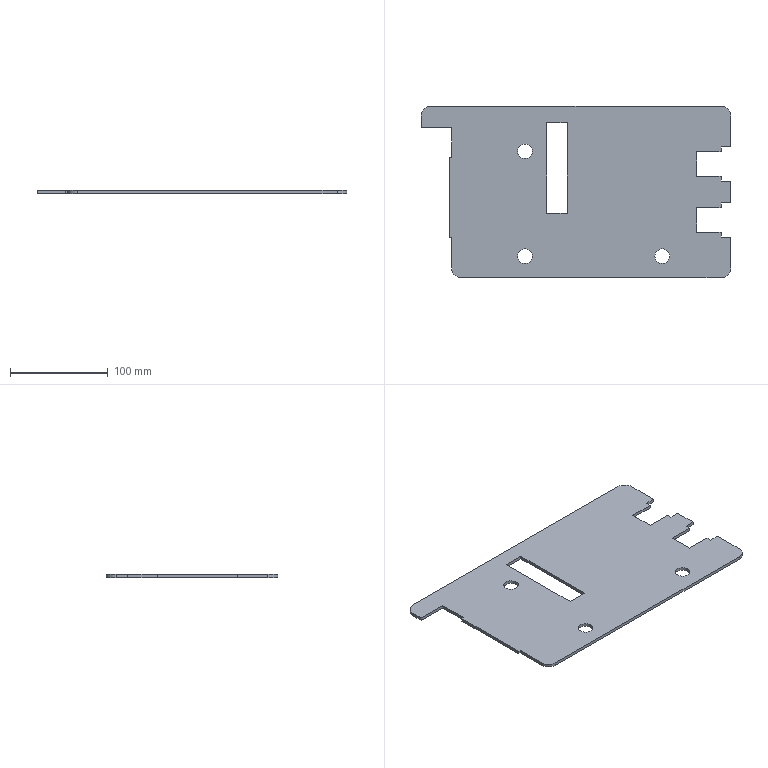Part | SolidWorks | features FlatPattern 1, SMBaseFlange 1, SheetMetal 1 | 1 solid | 42 faces | box 316 x 175 x 3.2 mm | volume 147992 mm3 | plane 32 | cylinder 10 | commonest cylinder face diameters 15 x6 20 x4
STEP:
#1=CARTESIAN_POINT('',(-77.5,-136.,3.2));
#2=VERTEX_POINT('',#1);
#3=CARTESIAN_POINT('',(-62.5,-136.,3.2));
#4=VERTEX_POINT('',#3);
#5=CARTESIAN_POINT('',(-70.,-136.,3.2));
#6=DIRECTION('',(0.,0.,1.));
#7=DIRECTION('',(1.,0.,0.));
#8=AXIS2_PLACEMENT_3D('',#5,#6,#7);
#9=CIRCLE('',#8,7.5);
#10=EDGE_CURVE('',#2,#4,#9,.T.);
#11=ORIENTED_EDGE('',*,*,#10,.T.);
#12=CARTESIAN_POINT('',(-62.5,-136.,0.));
#13=VERTEX_POINT('',#12);
#14=CARTESIAN_POINT('',(-62.5,-136.,3.2));
#15=DIRECTION('',(0.,0.,-1.));
#16=VECTOR('',#15,1000.);
#17=LINE('',#14,#16);
#18=EDGE_CURVE('',#4,#13,#17,.T.);
#19=ORIENTED_EDGE('',*,*,#18,.T.);
#20=CARTESIAN_POINT('',(-77.5,-136.,0.));
#21=VERTEX_POINT('',#20);
#22=CARTESIAN_POINT('',(-70.,-136.,0.));
#23=DIRECTION('',(0.,0.,1.));
#24=DIRECTION('',(1.,0.,0.));
#25=AXIS2_PLACEMENT_3D('',#22,#23,#24);
#26=CIRCLE('',#25,7.5);
#27=EDGE_CURVE('',#21,#13,#26,.T.);
#28=ORIENTED_EDGE('',*,*,#27,.F.);
#29=CARTESIAN_POINT('',(-77.5,-136.,3.2));
#30=DIRECTION('',(0.,0.,-1.));
#31=VECTOR('',#30,1000.);
#32=LINE('',#29,#31);
#33=EDGE_CURVE('',#2,#21,#32,.T.);
#34=ORIENTED_EDGE('',*,*,#33,.F.);
#35=EDGE_LOOP('',(#11,#19,#28,#34));
#36=FACE_OUTER_BOUND('',#35,.T.);
#37=CARTESIAN_POINT('',(-70.,-136.,3.2));
#38=DIRECTION('',(0.,0.,-1.));
#39=DIRECTION('',(-1.,0.,0.));
#40=AXIS2_PLACEMENT_3D('',#37,#38,#39);
#41=CYLINDRICAL_SURFACE('',#40,7.5);
#42=ADVANCED_FACE('',(#36),#41,.F.);
#43=CARTESIAN_POINT('',(-217.5,-136.,3.2));
#44=VERTEX_POINT('',#43);
#45=CARTESIAN_POINT('',(-202.5,-136.,3.2));
#46=VERTEX_POINT('',#45);
#47=CARTESIAN_POINT('',(-210.,-136.,3.2));
#48=DIRECTION('',(0.,0.,1.));
#49=DIRECTION('',(1.,0.,0.));
#50=AXIS2_PLACEMENT_3D('',#47,#48,#49);
#51=CIRCLE('',#50,7.5);
#52=EDGE_CURVE('',#44,#46,#51,.T.);
#53=ORIENTED_EDGE('',*,*,#52,.T.);
#54=CARTESIAN_POINT('',(-202.5,-136.,0.));
#55=VERTEX_POINT('',#54);
#56=CARTESIAN_POINT('',(-202.5,-136.,3.2));
#57=DIRECTION('',(0.,0.,-1.));
#58=VECTOR('',#57,1000.);
#59=LINE('',#56,#58);
#60=EDGE_CURVE('',#46,#55,#59,.T.);
#61=ORIENTED_EDGE('',*,*,#60,.T.);
#62=CARTESIAN_POINT('',(-217.5,-136.,0.));
#63=VERTEX_POINT('',#62);
#64=CARTESIAN_POINT('',(-210.,-136.,0.));
#65=DIRECTION('',(0.,0.,1.));
#66=DIRECTION('',(1.,0.,0.));
#67=AXIS2_PLACEMENT_3D('',#64,#65,#66);
#68=CIRCLE('',#67,7.5);
#69=EDGE_CURVE('',#63,#55,#68,.T.);
#70=ORIENTED_EDGE('',*,*,#69,.F.);
#71=CARTESIAN_POINT('',(-217.5,-136.,3.2));
#72=DIRECTION('',(0.,0.,-1.));
#73=VECTOR('',#72,1000.);
#74=LINE('',#71,#73);
#75=EDGE_CURVE('',#44,#63,#74,.T.);
#76=ORIENTED_EDGE('',*,*,#75,.F.);
#77=EDGE_LOOP('',(#53,#61,#70,#76));
#78=FACE_OUTER_BOUND('',#77,.T.);
#79=CARTESIAN_POINT('',(-210.,-136.,3.2));
#80=DIRECTION('',(0.,0.,-1.));
#81=DIRECTION('',(-1.,0.,0.));
#82=AXIS2_PLACEMENT_3D('',#79,#80,#81);
#83=CYLINDRICAL_SURFACE('',#82,7.5);
#84=ADVANCED_FACE('',(#78),#83,.F.);
#85=CARTESIAN_POINT('',(-217.5,-29.,3.2));
#86=VERTEX_POINT('',#85);
#87=CARTESIAN_POINT('',(-202.5,-29.,3.2));
#88=VERTEX_POINT('',#87);
#89=CARTESIAN_POINT('',(-210.,-29.,3.2));
#90=DIRECTION('',(0.,0.,1.));
#91=DIRECTION('',(1.,0.,0.));
#92=AXIS2_PLACEMENT_3D('',#89,#90,#91);
#93=CIRCLE('',#92,7.5);
#94=EDGE_CURVE('',#86,#88,#93,.T.);
#95=ORIENTED_EDGE('',*,*,#94,.T.);
#96=CARTESIAN_POINT('',(-202.5,-29.,0.));
#97=VERTEX_POINT('',#96);
#98=CARTESIAN_POINT('',(-202.5,-29.,3.2));
#99=DIRECTION('',(0.,0.,-1.));
#100=VECTOR('',#99,1000.);
#101=LINE('',#98,#100);
#102=EDGE_CURVE('',#88,#97,#101,.T.);
#103=ORIENTED_EDGE('',*,*,#102,.T.);
#104=CARTESIAN_POINT('',(-217.5,-29.,0.));
#105=VERTEX_POINT('',#104);
#106=CARTESIAN_POINT('',(-210.,-29.,0.));
#107=DIRECTION('',(0.,0.,1.));
#108=DIRECTION('',(1.,0.,0.));
#109=AXIS2_PLACEMENT_3D('',#106,#107,#108);
#110=CIRCLE('',#109,7.5);
#111=EDGE_CURVE('',#105,#97,#110,.T.);
#112=ORIENTED_EDGE('',*,*,#111,.F.);
#113=CARTESIAN_POINT('',(-217.5,-29.,3.2));
#114=DIRECTION('',(0.,0.,-1.));
#115=VECTOR('',#114,1000.);
#116=LINE('',#113,#115);
#117=EDGE_CURVE('',#86,#105,#116,.T.);
#118=ORIENTED_EDGE('',*,*,#117,.F.);
#119=EDGE_LOOP('',(#95,#103,#112,#118));
#120=FACE_OUTER_BOUND('',#119,.T.);
#121=CARTESIAN_POINT('',(-210.,-29.,3.2));
#122=DIRECTION('',(0.,0.,-1.));
#123=DIRECTION('',(-1.,0.,0.));
#124=AXIS2_PLACEMENT_3D('',#121,#122,#123);
#125=CYLINDRICAL_SURFACE('',#124,7.5);
#126=ADVANCED_FACE('',(#120),#125,.F.);
#127=ORIENTED_EDGE('',*,*,#10,.F.);
#128=CARTESIAN_POINT('',(-70.,-136.,3.2));
#129=DIRECTION('',(0.,0.,1.));
#130=DIRECTION('',(1.,0.,0.));
#131=AXIS2_PLACEMENT_3D('',#128,#129,#130);
#132=CIRCLE('',#131,7.5);
#133=EDGE_CURVE('',#4,#2,#132,.T.);
#134=ORIENTED_EDGE('',*,*,#133,.F.);
#135=EDGE_LOOP('',(#127,#134));
#136=FACE_BOUND('',#135,.T.);
#137=ORIENTED_EDGE('',*,*,#52,.F.);
#138=CARTESIAN_POINT('',(-210.,-136.,3.2));
#139=DIRECTION('',(0.,0.,1.));
#140=DIRECTION('',(1.,0.,0.));
#141=AXIS2_PLACEMENT_3D('',#138,#139,#140);
#142=CIRCLE('',#141,7.5);
#143=EDGE_CURVE('',#46,#44,#142,.T.);
#144=ORIENTED_EDGE('',*,*,#143,.F.);
#145=EDGE_LOOP('',(#137,#144));
#146=FACE_BOUND('',#145,.T.);
#147=ORIENTED_EDGE('',*,*,#94,.F.);
#148=CARTESIAN_POINT('',(-210.,-29.,3.2));
#149=DIRECTION('',(0.,0.,1.));
#150=DIRECTION('',(1.,0.,0.));
#151=AXIS2_PLACEMENT_3D('',#148,#149,#150);
#152=CIRCLE('',#151,7.5);
#153=EDGE_CURVE('',#88,#86,#152,.T.);
#154=ORIENTED_EDGE('',*,*,#153,.F.);
#155=EDGE_LOOP('',(#147,#154));
#156=FACE_BOUND('',#155,.T.);
#157=CARTESIAN_POINT('',(-285.,-148.,3.2));
#158=VERTEX_POINT('',#157);
#159=CARTESIAN_POINT('',(-275.,-158.,3.2));
#160=VERTEX_POINT('',#159);
#161=CARTESIAN_POINT('',(-275.,-148.,3.2));
#162=DIRECTION('',(0.,0.,1.));
#163=DIRECTION('',(-1.,0.,0.));
#164=AXIS2_PLACEMENT_3D('',#161,#162,#163);
#165=CIRCLE('',#164,10.);
#166=EDGE_CURVE('',#158,#160,#165,.T.);
#167=ORIENTED_EDGE('',*,*,#166,.T.);
#168=CARTESIAN_POINT('',(-10.,-158.,3.2));
#169=VERTEX_POINT('',#168);
#170=CARTESIAN_POINT('',(-275.,-158.,3.2));
#171=DIRECTION('',(1.,0.,0.));
#172=VECTOR('',#171,1000.);
#173=LINE('',#170,#172);
#174=EDGE_CURVE('',#160,#169,#173,.T.);
#175=ORIENTED_EDGE('',*,*,#174,.T.);
#176=CARTESIAN_POINT('',(0.,-148.,3.2));
#177=VERTEX_POINT('',#176);
#178=CARTESIAN_POINT('',(-10.,-148.,3.2));
#179=DIRECTION('',(0.,0.,1.));
#180=DIRECTION('',(1.,0.,0.));
#181=AXIS2_PLACEMENT_3D('',#178,#179,#180);
#182=CIRCLE('',#181,10.);
#183=EDGE_CURVE('',#169,#177,#182,.T.);
#184=ORIENTED_EDGE('',*,*,#183,.T.);
#185=CARTESIAN_POINT('',(0.,-116.5,3.2));
#186=VERTEX_POINT('',#185);
#187=CARTESIAN_POINT('',(0.,-148.,3.2));
#188=DIRECTION('',(0.,1.,0.));
#189=VECTOR('',#188,1000.);
#190=LINE('',#187,#189);
#191=EDGE_CURVE('',#177,#186,#190,.T.);
#192=ORIENTED_EDGE('',*,*,#191,.T.);
#193=CARTESIAN_POINT('',(-10.,-116.5,3.2));
#194=VERTEX_POINT('',#193);
#195=CARTESIAN_POINT('',(-10.,-116.5,3.2));
#196=DIRECTION('',(-1.,0.,0.));
#197=VECTOR('',#196,1000.);
#198=LINE('',#195,#197);
#199=EDGE_CURVE('',#186,#194,#198,.T.);
#200=ORIENTED_EDGE('',*,*,#199,.T.);
#201=CARTESIAN_POINT('',(-10.,-111.5,3.2));
#202=VERTEX_POINT('',#201);
#203=CARTESIAN_POINT('',(-10.,-111.5,3.2));
#204=DIRECTION('',(0.,1.,0.));
#205=VECTOR('',#204,1000.);
#206=LINE('',#203,#205);
#207=EDGE_CURVE('',#194,#202,#206,.T.);
#208=ORIENTED_EDGE('',*,*,#207,.T.);
#209=CARTESIAN_POINT('',(-35.,-111.5,3.2));
#210=VERTEX_POINT('',#209);
#211=CARTESIAN_POINT('',(-35.,-111.5,3.2));
#212=DIRECTION('',(-1.,0.,0.));
#213=VECTOR('',#212,1000.);
#214=LINE('',#211,#213);
#215=EDGE_CURVE('',#202,#210,#214,.T.);
#216=ORIENTED_EDGE('',*,*,#215,.T.);
#217=CARTESIAN_POINT('',(-35.,-86.5,3.2));
#218=VERTEX_POINT('',#217);
#219=CARTESIAN_POINT('',(-35.,-111.5,3.2));
#220=DIRECTION('',(0.,1.,0.));
#221=VECTOR('',#220,1000.);
#222=LINE('',#219,#221);
#223=EDGE_CURVE('',#210,#218,#222,.T.);
#224=ORIENTED_EDGE('',*,*,#223,.T.);
#225=CARTESIAN_POINT('',(-10.,-86.5,3.2));
#226=VERTEX_POINT('',#225);
#227=CARTESIAN_POINT('',(-35.,-86.5,3.2));
#228=DIRECTION('',(1.,0.,0.));
#229=VECTOR('',#228,1000.);
#230=LINE('',#227,#229);
#231=EDGE_CURVE('',#218,#226,#230,.T.);
#232=ORIENTED_EDGE('',*,*,#231,.T.);
#233=CARTESIAN_POINT('',(-10.,-81.5,3.2));
#234=VERTEX_POINT('',#233);
#235=CARTESIAN_POINT('',(-10.,-86.5,3.2));
#236=DIRECTION('',(0.,1.,0.));
#237=VECTOR('',#236,1000.);
#238=LINE('',#235,#237);
#239=EDGE_CURVE('',#226,#234,#238,.T.);
#240=ORIENTED_EDGE('',*,*,#239,.T.);
#241=CARTESIAN_POINT('',(0.,-81.5,3.2));
#242=VERTEX_POINT('',#241);
#243=CARTESIAN_POINT('',(-10.,-81.5,3.2));
#244=DIRECTION('',(1.,0.,0.));
#245=VECTOR('',#244,1000.);
#246=LINE('',#243,#245);
#247=EDGE_CURVE('',#234,#242,#246,.T.);
#248=ORIENTED_EDGE('',*,*,#247,.T.);
#249=CARTESIAN_POINT('',(0.,-59.5,3.2));
#250=VERTEX_POINT('',#249);
#251=CARTESIAN_POINT('',(0.,-81.5,3.2));
#252=DIRECTION('',(0.,1.,0.));
#253=VECTOR('',#252,1000.);
#254=LINE('',#251,#253);
#255=EDGE_CURVE('',#242,#250,#254,.T.);
#256=ORIENTED_EDGE('',*,*,#255,.T.);
#257=CARTESIAN_POINT('',(-10.,-59.5,3.2));
#258=VERTEX_POINT('',#257);
#259=CARTESIAN_POINT('',(-10.,-59.5,3.2));
#260=DIRECTION('',(-1.,0.,0.));
#261=VECTOR('',#260,1000.);
#262=LINE('',#259,#261);
#263=EDGE_CURVE('',#250,#258,#262,.T.);
#264=ORIENTED_EDGE('',*,*,#263,.T.);
#265=CARTESIAN_POINT('',(-10.,-54.5,3.2));
#266=VERTEX_POINT('',#265);
#267=CARTESIAN_POINT('',(-10.,-54.5,3.2));
#268=DIRECTION('',(0.,1.,0.));
#269=VECTOR('',#268,1000.);
#270=LINE('',#267,#269);
#271=EDGE_CURVE('',#258,#266,#270,.T.);
#272=ORIENTED_EDGE('',*,*,#271,.T.);
#273=CARTESIAN_POINT('',(-35.,-54.5,3.2));
#274=VERTEX_POINT('',#273);
#275=CARTESIAN_POINT('',(-35.,-54.5,3.2));
#276=DIRECTION('',(-1.,0.,0.));
#277=VECTOR('',#276,1000.);
#278=LINE('',#275,#277);
#279=EDGE_CURVE('',#266,#274,#278,.T.);
#280=ORIENTED_EDGE('',*,*,#279,.T.);
#281=CARTESIAN_POINT('',(-35.,-29.5,3.2));
#282=VERTEX_POINT('',#281);
#283=CARTESIAN_POINT('',(-35.,-54.5,3.2));
#284=DIRECTION('',(0.,1.,0.));
#285=VECTOR('',#284,1000.);
#286=LINE('',#283,#285);
#287=EDGE_CURVE('',#274,#282,#286,.T.);
#288=ORIENTED_EDGE('',*,*,#287,.T.);
#289=CARTESIAN_POINT('',(-10.,-29.5,3.2));
#290=VERTEX_POINT('',#289);
#291=CARTESIAN_POINT('',(-35.,-29.5,3.2));
#292=DIRECTION('',(1.,0.,0.));
#293=VECTOR('',#292,1000.);
#294=LINE('',#291,#293);
#295=EDGE_CURVE('',#282,#290,#294,.T.);
#296=ORIENTED_EDGE('',*,*,#295,.T.);
#297=CARTESIAN_POINT('',(-10.,-24.5,3.2));
#298=VERTEX_POINT('',#297);
#299=CARTESIAN_POINT('',(-10.,-29.5,3.2));
#300=DIRECTION('',(0.,1.,0.));
#301=VECTOR('',#300,1000.);
#302=LINE('',#299,#301);
#303=EDGE_CURVE('',#290,#298,#302,.T.);
#304=ORIENTED_EDGE('',*,*,#303,.T.);
#305=CARTESIAN_POINT('',(0.,-24.5,3.2));
#306=VERTEX_POINT('',#305);
#307=CARTESIAN_POINT('',(-10.,-24.5,3.2));
#308=DIRECTION('',(1.,0.,0.));
#309=VECTOR('',#308,1000.);
#310=LINE('',#307,#309);
#311=EDGE_CURVE('',#298,#306,#310,.T.);
#312=ORIENTED_EDGE('',*,*,#311,.T.);
#313=CARTESIAN_POINT('',(0.,7.,3.2));
#314=VERTEX_POINT('',#313);
#315=CARTESIAN_POINT('',(0.,-24.5,3.2));
#316=DIRECTION('',(0.,1.,0.));
#317=VECTOR('',#316,1000.);
#318=LINE('',#315,#317);
#319=EDGE_CURVE('',#306,#314,#318,.T.);
#320=ORIENTED_EDGE('',*,*,#319,.T.);
#321=CARTESIAN_POINT('',(-10.,17.,3.2));
#322=VERTEX_POINT('',#321);
#323=CARTESIAN_POINT('',(-10.,7.,3.2));
#324=DIRECTION('',(0.,0.,1.));
#325=DIRECTION('',(1.,0.,0.));
#326=AXIS2_PLACEMENT_3D('',#323,#324,#325);
#327=CIRCLE('',#326,10.);
#328=EDGE_CURVE('',#314,#322,#327,.T.);
#329=ORIENTED_EDGE('',*,*,#328,.T.);
#330=CARTESIAN_POINT('',(-306.,17.,3.2));
#331=VERTEX_POINT('',#330);
#332=CARTESIAN_POINT('',(-10.,17.,3.2));
#333=DIRECTION('',(-1.,0.,0.));
#334=VECTOR('',#333,1000.);
#335=LINE('',#332,#334);
#336=EDGE_CURVE('',#322,#331,#335,.T.);
#337=ORIENTED_EDGE('',*,*,#336,.T.);
#338=CARTESIAN_POINT('',(-316.,7.,3.2));
#339=VERTEX_POINT('',#338);
#340=CARTESIAN_POINT('',(-306.,7.,3.2));
#341=DIRECTION('',(0.,0.,1.));
#342=DIRECTION('',(1.,0.,0.));
#343=AXIS2_PLACEMENT_3D('',#340,#341,#342);
#344=CIRCLE('',#343,10.);
#345=EDGE_CURVE('',#331,#339,#344,.T.);
#346=ORIENTED_EDGE('',*,*,#345,.T.);
#347=CARTESIAN_POINT('',(-316.,-5.,3.2));
#348=VERTEX_POINT('',#347);
#349=CARTESIAN_POINT('',(-316.,7.,3.2));
#350=DIRECTION('',(0.,-1.,0.));
#351=VECTOR('',#350,1000.);
#352=LINE('',#349,#351);
#353=EDGE_CURVE('',#339,#348,#352,.T.);
#354=ORIENTED_EDGE('',*,*,#353,.T.);
#355=CARTESIAN_POINT('',(-285.,-5.,3.2));
#356=VERTEX_POINT('',#355);
#357=CARTESIAN_POINT('',(-316.,-5.,3.2));
#358=DIRECTION('',(1.,0.,0.));
#359=VECTOR('',#358,1000.);
#360=LINE('',#357,#359);
#361=EDGE_CURVE('',#348,#356,#360,.T.);
#362=ORIENTED_EDGE('',*,*,#361,.T.);
#363=CARTESIAN_POINT('',(-285.,-35.,3.2));
#364=VERTEX_POINT('',#363);
#365=CARTESIAN_POINT('',(-285.,-35.,3.2));
#366=DIRECTION('',(0.,-1.,0.));
#367=VECTOR('',#366,1000.);
#368=LINE('',#365,#367);
#369=EDGE_CURVE('',#356,#364,#368,.T.);
#370=ORIENTED_EDGE('',*,*,#369,.T.);
#371=CARTESIAN_POINT('',(-287.3,-35.,3.2));
#372=VERTEX_POINT('',#371);
#373=CARTESIAN_POINT('',(-285.,-35.,3.2));
#374=DIRECTION('',(-1.,0.,0.));
#375=VECTOR('',#374,1000.);
#376=LINE('',#373,#375);
#377=EDGE_CURVE('',#364,#372,#376,.T.);
#378=ORIENTED_EDGE('',*,*,#377,.T.);
#379=CARTESIAN_POINT('',(-287.3,-117.,3.2));
#380=VERTEX_POINT('',#379);
#381=CARTESIAN_POINT('',(-287.3,-35.,3.2));
#382=DIRECTION('',(0.,-1.,0.));
#383=VECTOR('',#382,1000.);
#384=LINE('',#381,#383);
#385=EDGE_CURVE('',#372,#380,#384,.T.);
#386=ORIENTED_EDGE('',*,*,#385,.T.);
#387=CARTESIAN_POINT('',(-285.,-117.,3.2));
#388=VERTEX_POINT('',#387);
#389=CARTESIAN_POINT('',(-287.3,-117.,3.2));
#390=DIRECTION('',(1.,0.,0.));
#391=VECTOR('',#390,1000.);
#392=LINE('',#389,#391);
#393=EDGE_CURVE('',#380,#388,#392,.T.);
#394=ORIENTED_EDGE('',*,*,#393,.T.);
#395=CARTESIAN_POINT('',(-285.,-148.,3.2));
#396=DIRECTION('',(0.,-1.,0.));
#397=VECTOR('',#396,1000.);
#398=LINE('',#395,#397);
#399=EDGE_CURVE('',#388,#158,#398,.T.);
#400=ORIENTED_EDGE('',*,*,#399,.T.);
#401=EDGE_LOOP('',(#167,#175,#184,#192,#200,#208,#216,#224,#232,#240,#248,#256,#264,#272,#280,#288,#296,#304,#312,#320,#329,#337,#346,#354,#362,#370,#378,#386,#394,#400));
#402=FACE_OUTER_BOUND('',#401,.T.);
#403=CARTESIAN_POINT('',(-188.,-92.,3.2));
#404=VERTEX_POINT('',#403);
#405=CARTESIAN_POINT('',(-167.,-92.,3.2));
#406=VERTEX_POINT('',#405);
#407=CARTESIAN_POINT('',(-167.,-92.,3.2));
#408=DIRECTION('',(1.,0.,0.));
#409=VECTOR('',#408,1000.);
#410=LINE('',#407,#409);
#411=EDGE_CURVE('',#404,#406,#410,.T.);
#412=ORIENTED_EDGE('',*,*,#411,.F.);
#413=CARTESIAN_POINT('',(-188.,0.,3.2));
#414=VERTEX_POINT('',#413);
#415=CARTESIAN_POINT('',(-188.,-92.,3.2));
#416=DIRECTION('',(0.,-1.,0.));
#417=VECTOR('',#416,1000.);
#418=LINE('',#415,#417);
#419=EDGE_CURVE('',#414,#404,#418,.T.);
#420=ORIENTED_EDGE('',*,*,#419,.F.);
#421=CARTESIAN_POINT('',(-167.,0.,3.2));
#422=VERTEX_POINT('',#421);
#423=CARTESIAN_POINT('',(-167.,0.,3.2));
#424=DIRECTION('',(-1.,0.,0.));
#425=VECTOR('',#424,1000.);
#426=LINE('',#423,#425);
#427=EDGE_CURVE('',#422,#414,#426,.T.);
#428=ORIENTED_EDGE('',*,*,#427,.F.);
#429=CARTESIAN_POINT('',(-167.,-92.,3.2));
#430=DIRECTION('',(0.,1.,0.));
#431=VECTOR('',#430,1000.);
#432=LINE('',#429,#431);
#433=EDGE_CURVE('',#406,#422,#432,.T.);
#434=ORIENTED_EDGE('',*,*,#433,.F.);
#435=EDGE_LOOP('',(#412,#420,#428,#434));
#436=FACE_BOUND('',#435,.T.);
#437=CARTESIAN_POINT('',(-275.,-148.,3.2));
#438=DIRECTION('',(0.,0.,-1.));
#439=DIRECTION('',(-1.,0.,0.));
#440=AXIS2_PLACEMENT_3D('',#437,#438,#439);
#441=PLANE('',#440);
#442=ADVANCED_FACE('',(#136,#146,#156,#402,#436),#441,.F.);
#443=ORIENTED_EDGE('',*,*,#69,.T.);
#444=CARTESIAN_POINT('',(-210.,-136.,0.));
#445=DIRECTION('',(0.,0.,1.));
#446=DIRECTION('',(1.,0.,0.));
#447=AXIS2_PLACEMENT_3D('',#444,#445,#446);
#448=CIRCLE('',#447,7.5);
#449=EDGE_CURVE('',#55,#63,#448,.T.);
#450=ORIENTED_EDGE('',*,*,#449,.T.);
#451=EDGE_LOOP('',(#443,#450));
#452=FACE_BOUND('',#451,.T.);
#453=CARTESIAN_POINT('',(-285.,-148.,0.));
#454=VERTEX_POINT('',#453);
#455=CARTESIAN_POINT('',(-275.,-158.,0.));
#456=VERTEX_POINT('',#455);
#457=CARTESIAN_POINT('',(-275.,-148.,0.));
#458=DIRECTION('',(0.,0.,1.));
#459=DIRECTION('',(-1.,0.,0.));
#460=AXIS2_PLACEMENT_3D('',#457,#458,#459);
#461=CIRCLE('',#460,10.);
#462=EDGE_CURVE('',#454,#456,#461,.T.);
#463=ORIENTED_EDGE('',*,*,#462,.F.);
#464=CARTESIAN_POINT('',(-285.,-117.,0.));
#465=VERTEX_POINT('',#464);
#466=CARTESIAN_POINT('',(-285.,-148.,0.));
#467=DIRECTION('',(0.,-1.,0.));
#468=VECTOR('',#467,1000.);
#469=LINE('',#466,#468);
#470=EDGE_CURVE('',#465,#454,#469,.T.);
#471=ORIENTED_EDGE('',*,*,#470,.F.);
#472=CARTESIAN_POINT('',(-287.3,-117.,0.));
#473=VERTEX_POINT('',#472);
#474=CARTESIAN_POINT('',(-287.3,-117.,0.));
#475=DIRECTION('',(1.,0.,0.));
#476=VECTOR('',#475,1000.);
#477=LINE('',#474,#476);
#478=EDGE_CURVE('',#473,#465,#477,.T.);
#479=ORIENTED_EDGE('',*,*,#478,.F.);
#480=CARTESIAN_POINT('',(-287.3,-35.,0.));
#481=VERTEX_POINT('',#480);
#482=CARTESIAN_POINT('',(-287.3,-35.,0.));
#483=DIRECTION('',(0.,-1.,0.));
#484=VECTOR('',#483,1000.);
#485=LINE('',#482,#484);
#486=EDGE_CURVE('',#481,#473,#485,.T.);
#487=ORIENTED_EDGE('',*,*,#486,.F.);
#488=CARTESIAN_POINT('',(-285.,-35.,0.));
#489=VERTEX_POINT('',#488);
#490=CARTESIAN_POINT('',(-285.,-35.,0.));
#491=DIRECTION('',(-1.,0.,0.));
#492=VECTOR('',#491,1000.);
#493=LINE('',#490,#492);
#494=EDGE_CURVE('',#489,#481,#493,.T.);
#495=ORIENTED_EDGE('',*,*,#494,.F.);
#496=CARTESIAN_POINT('',(-285.,-5.,0.));
#497=VERTEX_POINT('',#496);
#498=CARTESIAN_POINT('',(-285.,-35.,0.));
#499=DIRECTION('',(0.,-1.,0.));
#500=VECTOR('',#499,1000.);
#501=LINE('',#498,#500);
#502=EDGE_CURVE('',#497,#489,#501,.T.);
#503=ORIENTED_EDGE('',*,*,#502,.F.);
#504=CARTESIAN_POINT('',(-316.,-5.,0.));
#505=VERTEX_POINT('',#504);
#506=CARTESIAN_POINT('',(-316.,-5.,0.));
#507=DIRECTION('',(1.,0.,0.));
#508=VECTOR('',#507,1000.);
#509=LINE('',#506,#508);
#510=EDGE_CURVE('',#505,#497,#509,.T.);
#511=ORIENTED_EDGE('',*,*,#510,.F.);
#512=CARTESIAN_POINT('',(-316.,7.,0.));
#513=VERTEX_POINT('',#512);
#514=CARTESIAN_POINT('',(-316.,7.,0.));
#515=DIRECTION('',(0.,-1.,0.));
#516=VECTOR('',#515,1000.);
#517=LINE('',#514,#516);
#518=EDGE_CURVE('',#513,#505,#517,.T.);
#519=ORIENTED_EDGE('',*,*,#518,.F.);
#520=CARTESIAN_POINT('',(-306.,17.,0.));
#521=VERTEX_POINT('',#520);
#522=CARTESIAN_POINT('',(-306.,7.,0.));
#523=DIRECTION('',(0.,0.,1.));
#524=DIRECTION('',(1.,0.,0.));
#525=AXIS2_PLACEMENT_3D('',#522,#523,#524);
#526=CIRCLE('',#525,10.);
#527=EDGE_CURVE('',#521,#513,#526,.T.);
#528=ORIENTED_EDGE('',*,*,#527,.F.);
#529=CARTESIAN_POINT('',(-10.,17.,0.));
#530=VERTEX_POINT('',#529);
#531=CARTESIAN_POINT('',(-10.,17.,0.));
#532=DIRECTION('',(-1.,0.,0.));
#533=VECTOR('',#532,1000.);
#534=LINE('',#531,#533);
#535=EDGE_CURVE('',#530,#521,#534,.T.);
#536=ORIENTED_EDGE('',*,*,#535,.F.);
#537=CARTESIAN_POINT('',(0.,7.,0.));
#538=VERTEX_POINT('',#537);
#539=CARTESIAN_POINT('',(-10.,7.,0.));
#540=DIRECTION('',(0.,0.,1.));
#541=DIRECTION('',(1.,0.,0.));
#542=AXIS2_PLACEMENT_3D('',#539,#540,#541);
#543=CIRCLE('',#542,10.);
#544=EDGE_CURVE('',#538,#530,#543,.T.);
#545=ORIENTED_EDGE('',*,*,#544,.F.);
#546=CARTESIAN_POINT('',(0.,-24.5,0.));
#547=VERTEX_POINT('',#546);
#548=CARTESIAN_POINT('',(0.,-24.5,0.));
#549=DIRECTION('',(0.,1.,0.));
#550=VECTOR('',#549,1000.);
#551=LINE('',#548,#550);
#552=EDGE_CURVE('',#547,#538,#551,.T.);
#553=ORIENTED_EDGE('',*,*,#552,.F.);
#554=CARTESIAN_POINT('',(-10.,-24.5,0.));
#555=VERTEX_POINT('',#554);
#556=CARTESIAN_POINT('',(-10.,-24.5,0.));
#557=DIRECTION('',(1.,0.,0.));
#558=VECTOR('',#557,1000.);
#559=LINE('',#556,#558);
#560=EDGE_CURVE('',#555,#547,#559,.T.);
#561=ORIENTED_EDGE('',*,*,#560,.F.);
#562=CARTESIAN_POINT('',(-10.,-29.5,0.));
#563=VERTEX_POINT('',#562);
#564=CARTESIAN_POINT('',(-10.,-29.5,0.));
#565=DIRECTION('',(0.,1.,0.));
#566=VECTOR('',#565,1000.);
#567=LINE('',#564,#566);
#568=EDGE_CURVE('',#563,#555,#567,.T.);
#569=ORIENTED_EDGE('',*,*,#568,.F.);
#570=CARTESIAN_POINT('',(-35.,-29.5,0.));
#571=VERTEX_POINT('',#570);
#572=CARTESIAN_POINT('',(-35.,-29.5,0.));
#573=DIRECTION('',(1.,0.,0.));
#574=VECTOR('',#573,1000.);
#575=LINE('',#572,#574);
#576=EDGE_CURVE('',#571,#563,#575,.T.);
#577=ORIENTED_EDGE('',*,*,#576,.F.);
#578=CARTESIAN_POINT('',(-35.,-54.5,0.));
#579=VERTEX_POINT('',#578);
#580=CARTESIAN_POINT('',(-35.,-54.5,0.));
#581=DIRECTION('',(0.,1.,0.));
#582=VECTOR('',#581,1000.);
#583=LINE('',#580,#582);
#584=EDGE_CURVE('',#579,#571,#583,.T.);
#585=ORIENTED_EDGE('',*,*,#584,.F.);
#586=CARTESIAN_POINT('',(-10.,-54.5,0.));
#587=VERTEX_POINT('',#586);
#588=CARTESIAN_POINT('',(-35.,-54.5,0.));
#589=DIRECTION('',(-1.,0.,0.));
#590=VECTOR('',#589,1000.);
#591=LINE('',#588,#590);
#592=EDGE_CURVE('',#587,#579,#591,.T.);
#593=ORIENTED_EDGE('',*,*,#592,.F.);
#594=CARTESIAN_POINT('',(-10.,-59.5,0.));
#595=VERTEX_POINT('',#594);
#596=CARTESIAN_POINT('',(-10.,-54.5,0.));
#597=DIRECTION('',(0.,1.,0.));
#598=VECTOR('',#597,1000.);
#599=LINE('',#596,#598);
#600=EDGE_CURVE('',#595,#587,#599,.T.);
#601=ORIENTED_EDGE('',*,*,#600,.F.);
#602=CARTESIAN_POINT('',(0.,-59.5,0.));
#603=VERTEX_POINT('',#602);
#604=CARTESIAN_POINT('',(-10.,-59.5,0.));
#605=DIRECTION('',(-1.,0.,0.));
#606=VECTOR('',#605,1000.);
#607=LINE('',#604,#606);
#608=EDGE_CURVE('',#603,#595,#607,.T.);
#609=ORIENTED_EDGE('',*,*,#608,.F.);
#610=CARTESIAN_POINT('',(0.,-81.5,0.));
#611=VERTEX_POINT('',#610);
#612=CARTESIAN_POINT('',(0.,-81.5,0.));
#613=DIRECTION('',(0.,1.,0.));
#614=VECTOR('',#613,1000.);
#615=LINE('',#612,#614);
#616=EDGE_CURVE('',#611,#603,#615,.T.);
#617=ORIENTED_EDGE('',*,*,#616,.F.);
#618=CARTESIAN_POINT('',(-10.,-81.5,0.));
#619=VERTEX_POINT('',#618);
#620=CARTESIAN_POINT('',(-10.,-81.5,0.));
#621=DIRECTION('',(1.,0.,0.));
#622=VECTOR('',#621,1000.);
#623=LINE('',#620,#622);
#624=EDGE_CURVE('',#619,#611,#623,.T.);
#625=ORIENTED_EDGE('',*,*,#624,.F.);
#626=CARTESIAN_POINT('',(-10.,-86.5,0.));
#627=VERTEX_POINT('',#626);
#628=CARTESIAN_POINT('',(-10.,-86.5,0.));
#629=DIRECTION('',(0.,1.,0.));
#630=VECTOR('',#629,1000.);
#631=LINE('',#628,#630);
#632=EDGE_CURVE('',#627,#619,#631,.T.);
#633=ORIENTED_EDGE('',*,*,#632,.F.);
#634=CARTESIAN_POINT('',(-35.,-86.5,0.));
#635=VERTEX_POINT('',#634);
#636=CARTESIAN_POINT('',(-35.,-86.5,0.));
#637=DIRECTION('',(1.,0.,0.));
#638=VECTOR('',#637,1000.);
#639=LINE('',#636,#638);
#640=EDGE_CURVE('',#635,#627,#639,.T.);
#641=ORIENTED_EDGE('',*,*,#640,.F.);
#642=CARTESIAN_POINT('',(-35.,-111.5,0.));
#643=VERTEX_POINT('',#642);
#644=CARTESIAN_POINT('',(-35.,-111.5,0.));
#645=DIRECTION('',(0.,1.,0.));
#646=VECTOR('',#645,1000.);
#647=LINE('',#644,#646);
#648=EDGE_CURVE('',#643,#635,#647,.T.);
#649=ORIENTED_EDGE('',*,*,#648,.F.);
#650=CARTESIAN_POINT('',(-10.,-111.5,0.));
#651=VERTEX_POINT('',#650);
#652=CARTESIAN_POINT('',(-35.,-111.5,0.));
#653=DIRECTION('',(-1.,0.,0.));
#654=VECTOR('',#653,1000.);
#655=LINE('',#652,#654);
#656=EDGE_CURVE('',#651,#643,#655,.T.);
#657=ORIENTED_EDGE('',*,*,#656,.F.);
#658=CARTESIAN_POINT('',(-10.,-116.5,0.));
#659=VERTEX_POINT('',#658);
#660=CARTESIAN_POINT('',(-10.,-111.5,0.));
#661=DIRECTION('',(0.,1.,0.));
#662=VECTOR('',#661,1000.);
#663=LINE('',#660,#662);
#664=EDGE_CURVE('',#659,#651,#663,.T.);
#665=ORIENTED_EDGE('',*,*,#664,.F.);
#666=CARTESIAN_POINT('',(0.,-116.5,0.));
#667=VERTEX_POINT('',#666);
#668=CARTESIAN_POINT('',(-10.,-116.5,0.));
#669=DIRECTION('',(-1.,0.,0.));
#670=VECTOR('',#669,1000.);
#671=LINE('',#668,#670);
#672=EDGE_CURVE('',#667,#659,#671,.T.);
#673=ORIENTED_EDGE('',*,*,#672,.F.);
#674=CARTESIAN_POINT('',(0.,-148.,0.));
#675=VERTEX_POINT('',#674);
#676=CARTESIAN_POINT('',(0.,-148.,0.));
#677=DIRECTION('',(0.,1.,0.));
#678=VECTOR('',#677,1000.);
#679=LINE('',#676,#678);
#680=EDGE_CURVE('',#675,#667,#679,.T.);
#681=ORIENTED_EDGE('',*,*,#680,.F.);
#682=CARTESIAN_POINT('',(-10.,-158.,0.));
#683=VERTEX_POINT('',#682);
#684=CARTESIAN_POINT('',(-10.,-148.,0.));
#685=DIRECTION('',(0.,0.,1.));
#686=DIRECTION('',(1.,0.,0.));
#687=AXIS2_PLACEMENT_3D('',#684,#685,#686);
#688=CIRCLE('',#687,10.);
#689=EDGE_CURVE('',#683,#675,#688,.T.);
#690=ORIENTED_EDGE('',*,*,#689,.F.);
#691=CARTESIAN_POINT('',(-275.,-158.,0.));
#692=DIRECTION('',(1.,0.,0.));
#693=VECTOR('',#692,1000.);
#694=LINE('',#691,#693);
#695=EDGE_CURVE('',#456,#683,#694,.T.);
#696=ORIENTED_EDGE('',*,*,#695,.F.);
#697=EDGE_LOOP('',(#463,#471,#479,#487,#495,#503,#511,#519,#528,#536,#545,#553,#561,#569,#577,#585,#593,#601,#609,#617,#625,#633,#641,#649,#657,#665,#673,#681,#690,#696));
#698=FACE_OUTER_BOUND('',#697,.T.);
#699=ORIENTED_EDGE('',*,*,#111,.T.);
#700=CARTESIAN_POINT('',(-210.,-29.,0.));
#701=DIRECTION('',(0.,0.,1.));
#702=DIRECTION('',(1.,0.,0.));
#703=AXIS2_PLACEMENT_3D('',#700,#701,#702);
#704=CIRCLE('',#703,7.5);
#705=EDGE_CURVE('',#97,#105,#704,.T.);
#706=ORIENTED_EDGE('',*,*,#705,.T.);
#707=EDGE_LOOP('',(#699,#706));
#708=FACE_BOUND('',#707,.T.);
#709=ORIENTED_EDGE('',*,*,#27,.T.);
#710=CARTESIAN_POINT('',(-70.,-136.,0.));
#711=DIRECTION('',(0.,0.,1.));
#712=DIRECTION('',(1.,0.,0.));
#713=AXIS2_PLACEMENT_3D('',#710,#711,#712);
#714=CIRCLE('',#713,7.5);
#715=EDGE_CURVE('',#13,#21,#714,.T.);
#716=ORIENTED_EDGE('',*,*,#715,.T.);
#717=EDGE_LOOP('',(#709,#716));
#718=FACE_BOUND('',#717,.T.);
#719=CARTESIAN_POINT('',(-188.,0.,0.));
#720=VERTEX_POINT('',#719);
#721=CARTESIAN_POINT('',(-188.,-92.,0.));
#722=VERTEX_POINT('',#721);
#723=CARTESIAN_POINT('',(-188.,-92.,0.));
#724=DIRECTION('',(0.,-1.,0.));
#725=VECTOR('',#724,1000.);
#726=LINE('',#723,#725);
#727=EDGE_CURVE('',#720,#722,#726,.T.);
#728=ORIENTED_EDGE('',*,*,#727,.T.);
#729=CARTESIAN_POINT('',(-167.,-92.,0.));
#730=VERTEX_POINT('',#729);
#731=CARTESIAN_POINT('',(-167.,-92.,0.));
#732=DIRECTION('',(1.,0.,0.));
#733=VECTOR('',#732,1000.);
#734=LINE('',#731,#733);
#735=EDGE_CURVE('',#722,#730,#734,.T.);
#736=ORIENTED_EDGE('',*,*,#735,.T.);
#737=CARTESIAN_POINT('',(-167.,0.,0.));
#738=VERTEX_POINT('',#737);
#739=CARTESIAN_POINT('',(-167.,-92.,0.));
#740=DIRECTION('',(0.,1.,0.));
#741=VECTOR('',#740,1000.);
#742=LINE('',#739,#741);
#743=EDGE_CURVE('',#730,#738,#742,.T.);
#744=ORIENTED_EDGE('',*,*,#743,.T.);
#745=CARTESIAN_POINT('',(-167.,0.,0.));
#746=DIRECTION('',(-1.,0.,0.));
#747=VECTOR('',#746,1000.);
#748=LINE('',#745,#747);
#749=EDGE_CURVE('',#738,#720,#748,.T.);
#750=ORIENTED_EDGE('',*,*,#749,.T.);
#751=EDGE_LOOP('',(#728,#736,#744,#750));
#752=FACE_BOUND('',#751,.T.);
#753=CARTESIAN_POINT('',(-275.,-148.,0.));
#754=DIRECTION('',(0.,0.,-1.));
#755=DIRECTION('',(-1.,0.,0.));
#756=AXIS2_PLACEMENT_3D('',#753,#754,#755);
#757=PLANE('',#756);
#758=ADVANCED_FACE('',(#452,#698,#708,#718,#752),#757,.T.);
#759=ORIENTED_EDGE('',*,*,#462,.T.);
#760=CARTESIAN_POINT('',(-275.,-158.,3.2));
#761=DIRECTION('',(0.,0.,-1.));
#762=VECTOR('',#761,1000.);
#763=LINE('',#760,#762);
#764=EDGE_CURVE('',#160,#456,#763,.T.);
#765=ORIENTED_EDGE('',*,*,#764,.F.);
#766=ORIENTED_EDGE('',*,*,#166,.F.);
#767=CARTESIAN_POINT('',(-285.,-148.,3.2));
#768=DIRECTION('',(0.,0.,-1.));
#769=VECTOR('',#768,1000.);
#770=LINE('',#767,#769);
#771=EDGE_CURVE('',#158,#454,#770,.T.);
#772=ORIENTED_EDGE('',*,*,#771,.T.);
#773=EDGE_LOOP('',(#759,#765,#766,#772));
#774=FACE_OUTER_BOUND('',#773,.T.);
#775=CARTESIAN_POINT('',(-275.,-148.,3.2));
#776=DIRECTION('',(0.,0.,-1.));
#777=DIRECTION('',(-1.,0.,0.));
#778=AXIS2_PLACEMENT_3D('',#775,#776,#777);
#779=CYLINDRICAL_SURFACE('',#778,10.);
#780=ADVANCED_FACE('',(#774),#779,.T.);
#781=ORIENTED_EDGE('',*,*,#695,.T.);
#782=CARTESIAN_POINT('',(-10.,-158.,3.2));
#783=DIRECTION('',(0.,0.,-1.));
#784=VECTOR('',#783,1000.);
#785=LINE('',#782,#784);
#786=EDGE_CURVE('',#169,#683,#785,.T.);
#787=ORIENTED_EDGE('',*,*,#786,.F.);
#788=ORIENTED_EDGE('',*,*,#174,.F.);
#789=ORIENTED_EDGE('',*,*,#764,.T.);
#790=EDGE_LOOP('',(#781,#787,#788,#789));
#791=FACE_OUTER_BOUND('',#790,.T.);
#792=CARTESIAN_POINT('',(-275.,-158.,3.2));
#793=DIRECTION('',(0.,1.,0.));
#794=DIRECTION('',(0.,0.,1.));
#795=AXIS2_PLACEMENT_3D('',#792,#793,#794);
#796=PLANE('',#795);
#797=ADVANCED_FACE('',(#791),#796,.F.);
#798=ORIENTED_EDGE('',*,*,#689,.T.);
#799=CARTESIAN_POINT('',(0.,-148.,3.2));
#800=DIRECTION('',(0.,0.,-1.));
#801=VECTOR('',#800,1000.);
#802=LINE('',#799,#801);
#803=EDGE_CURVE('',#177,#675,#802,.T.);
#804=ORIENTED_EDGE('',*,*,#803,.F.);
#805=ORIENTED_EDGE('',*,*,#183,.F.);
#806=ORIENTED_EDGE('',*,*,#786,.T.);
#807=EDGE_LOOP('',(#798,#804,#805,#806));
#808=FACE_OUTER_BOUND('',#807,.T.);
#809=CARTESIAN_POINT('',(-10.,-148.,3.2));
#810=DIRECTION('',(0.,0.,-1.));
#811=DIRECTION('',(-1.,0.,0.));
#812=AXIS2_PLACEMENT_3D('',#809,#810,#811);
#813=CYLINDRICAL_SURFACE('',#812,10.);
#814=ADVANCED_FACE('',(#808),#813,.T.);
#815=ORIENTED_EDGE('',*,*,#680,.T.);
#816=CARTESIAN_POINT('',(0.,-116.5,3.2));
#817=DIRECTION('',(0.,0.,-1.));
#818=VECTOR('',#817,1000.);
#819=LINE('',#816,#818);
#820=EDGE_CURVE('',#186,#667,#819,.T.);
#821=ORIENTED_EDGE('',*,*,#820,.F.);
#822=ORIENTED_EDGE('',*,*,#191,.F.);
#823=ORIENTED_EDGE('',*,*,#803,.T.);
#824=EDGE_LOOP('',(#815,#821,#822,#823));
#825=FACE_OUTER_BOUND('',#824,.T.);
#826=CARTESIAN_POINT('',(0.,-148.,3.2));
#827=DIRECTION('',(-1.,0.,0.));
#828=DIRECTION('',(0.,-1.,0.));
#829=AXIS2_PLACEMENT_3D('',#826,#827,#828);
#830=PLANE('',#829);
#831=ADVANCED_FACE('',(#825),#830,.F.);
#832=ORIENTED_EDGE('',*,*,#672,.T.);
#833=CARTESIAN_POINT('',(-10.,-116.5,3.2));
#834=DIRECTION('',(0.,0.,-1.));
#835=VECTOR('',#834,1000.);
#836=LINE('',#833,#835);
#837=EDGE_CURVE('',#194,#659,#836,.T.);
#838=ORIENTED_EDGE('',*,*,#837,.F.);
#839=ORIENTED_EDGE('',*,*,#199,.F.);
#840=ORIENTED_EDGE('',*,*,#820,.T.);
#841=EDGE_LOOP('',(#832,#838,#839,#840));
#842=FACE_OUTER_BOUND('',#841,.T.);
#843=CARTESIAN_POINT('',(-10.,-116.5,3.2));
#844=DIRECTION('',(0.,-1.,0.));
#845=DIRECTION('',(0.,0.,-1.));
#846=AXIS2_PLACEMENT_3D('',#843,#844,#845);
#847=PLANE('',#846);
#848=ADVANCED_FACE('',(#842),#847,.F.);
#849=ORIENTED_EDGE('',*,*,#664,.T.);
#850=CARTESIAN_POINT('',(-10.,-111.5,3.2));
#851=DIRECTION('',(0.,0.,-1.));
#852=VECTOR('',#851,1000.);
#853=LINE('',#850,#852);
#854=EDGE_CURVE('',#202,#651,#853,.T.);
#855=ORIENTED_EDGE('',*,*,#854,.F.);
#856=ORIENTED_EDGE('',*,*,#207,.F.);
#857=ORIENTED_EDGE('',*,*,#837,.T.);
#858=EDGE_LOOP('',(#849,#855,#856,#857));
#859=FACE_OUTER_BOUND('',#858,.T.);
#860=CARTESIAN_POINT('',(-10.,-111.5,3.2));
#861=DIRECTION('',(-1.,0.,0.));
#862=DIRECTION('',(0.,-1.,0.));
#863=AXIS2_PLACEMENT_3D('',#860,#861,#862);
#864=PLANE('',#863);
#865=ADVANCED_FACE('',(#859),#864,.F.);
#866=ORIENTED_EDGE('',*,*,#656,.T.);
#867=CARTESIAN_POINT('',(-35.,-111.5,3.2));
#868=DIRECTION('',(0.,0.,-1.));
#869=VECTOR('',#868,1000.);
#870=LINE('',#867,#869);
#871=EDGE_CURVE('',#210,#643,#870,.T.);
#872=ORIENTED_EDGE('',*,*,#871,.F.);
#873=ORIENTED_EDGE('',*,*,#215,.F.);
#874=ORIENTED_EDGE('',*,*,#854,.T.);
#875=EDGE_LOOP('',(#866,#872,#873,#874));
#876=FACE_OUTER_BOUND('',#875,.T.);
#877=CARTESIAN_POINT('',(-35.,-111.5,3.2));
#878=DIRECTION('',(0.,-1.,0.));
#879=DIRECTION('',(0.,0.,-1.));
#880=AXIS2_PLACEMENT_3D('',#877,#878,#879);
#881=PLANE('',#880);
#882=ADVANCED_FACE('',(#876),#881,.F.);
#883=ORIENTED_EDGE('',*,*,#648,.T.);
#884=CARTESIAN_POINT('',(-35.,-86.5,3.2));
#885=DIRECTION('',(0.,0.,-1.));
#886=VECTOR('',#885,1000.);
#887=LINE('',#884,#886);
#888=EDGE_CURVE('',#218,#635,#887,.T.);
#889=ORIENTED_EDGE('',*,*,#888,.F.);
#890=ORIENTED_EDGE('',*,*,#223,.F.);
#891=ORIENTED_EDGE('',*,*,#871,.T.);
#892=EDGE_LOOP('',(#883,#889,#890,#891));
#893=FACE_OUTER_BOUND('',#892,.T.);
#894=CARTESIAN_POINT('',(-35.,-111.5,3.2));
#895=DIRECTION('',(-1.,0.,0.));
#896=DIRECTION('',(0.,0.,1.));
#897=AXIS2_PLACEMENT_3D('',#894,#895,#896);
#898=PLANE('',#897);
#899=ADVANCED_FACE('',(#893),#898,.F.);
#900=ORIENTED_EDGE('',*,*,#640,.T.);
#901=CARTESIAN_POINT('',(-10.,-86.5,3.2));
#902=DIRECTION('',(0.,0.,-1.));
#903=VECTOR('',#902,1000.);
#904=LINE('',#901,#903);
#905=EDGE_CURVE('',#226,#627,#904,.T.);
#906=ORIENTED_EDGE('',*,*,#905,.F.);
#907=ORIENTED_EDGE('',*,*,#231,.F.);
#908=ORIENTED_EDGE('',*,*,#888,.T.);
#909=EDGE_LOOP('',(#900,#906,#907,#908));
#910=FACE_OUTER_BOUND('',#909,.T.);
#911=CARTESIAN_POINT('',(-35.,-86.5,3.2));
#912=DIRECTION('',(0.,1.,0.));
#913=DIRECTION('',(0.,0.,1.));
#914=AXIS2_PLACEMENT_3D('',#911,#912,#913);
#915=PLANE('',#914);
#916=ADVANCED_FACE('',(#910),#915,.F.);
#917=ORIENTED_EDGE('',*,*,#632,.T.);
#918=CARTESIAN_POINT('',(-10.,-81.5,3.2));
#919=DIRECTION('',(0.,0.,-1.));
#920=VECTOR('',#919,1000.);
#921=LINE('',#918,#920);
#922=EDGE_CURVE('',#234,#619,#921,.T.);
#923=ORIENTED_EDGE('',*,*,#922,.F.);
#924=ORIENTED_EDGE('',*,*,#239,.F.);
#925=ORIENTED_EDGE('',*,*,#905,.T.);
#926=EDGE_LOOP('',(#917,#923,#924,#925));
#927=FACE_OUTER_BOUND('',#926,.T.);
#928=CARTESIAN_POINT('',(-10.,-86.5,3.2));
#929=DIRECTION('',(-1.,0.,0.));
#930=DIRECTION('',(0.,-1.,0.));
#931=AXIS2_PLACEMENT_3D('',#928,#929,#930);
#932=PLANE('',#931);
#933=ADVANCED_FACE('',(#927),#932,.F.);
#934=ORIENTED_EDGE('',*,*,#624,.T.);
#935=CARTESIAN_POINT('',(0.,-81.5,3.2));
#936=DIRECTION('',(0.,0.,-1.));
#937=VECTOR('',#936,1000.);
#938=LINE('',#935,#937);
#939=EDGE_CURVE('',#242,#611,#938,.T.);
#940=ORIENTED_EDGE('',*,*,#939,.F.);
#941=ORIENTED_EDGE('',*,*,#247,.F.);
#942=ORIENTED_EDGE('',*,*,#922,.T.);
#943=EDGE_LOOP('',(#934,#940,#941,#942));
#944=FACE_OUTER_BOUND('',#943,.T.);
#945=CARTESIAN_POINT('',(-10.,-81.5,3.2));
#946=DIRECTION('',(0.,1.,0.));
#947=DIRECTION('',(0.,0.,1.));
#948=AXIS2_PLACEMENT_3D('',#945,#946,#947);
#949=PLANE('',#948);
#950=ADVANCED_FACE('',(#944),#949,.F.);
#951=ORIENTED_EDGE('',*,*,#616,.T.);
#952=CARTESIAN_POINT('',(0.,-59.5,3.2));
#953=DIRECTION('',(0.,0.,-1.));
#954=VECTOR('',#953,1000.);
#955=LINE('',#952,#954);
#956=EDGE_CURVE('',#250,#603,#955,.T.);
#957=ORIENTED_EDGE('',*,*,#956,.F.);
#958=ORIENTED_EDGE('',*,*,#255,.F.);
#959=ORIENTED_EDGE('',*,*,#939,.T.);
#960=EDGE_LOOP('',(#951,#957,#958,#959));
#961=FACE_OUTER_BOUND('',#960,.T.);
#962=CARTESIAN_POINT('',(0.,-81.5,3.2));
#963=DIRECTION('',(-1.,0.,0.));
#964=DIRECTION('',(0.,-1.,0.));
#965=AXIS2_PLACEMENT_3D('',#962,#963,#964);
#966=PLANE('',#965);
#967=ADVANCED_FACE('',(#961),#966,.F.);
#968=ORIENTED_EDGE('',*,*,#608,.T.);
#969=CARTESIAN_POINT('',(-10.,-59.5,3.2));
#970=DIRECTION('',(0.,0.,-1.));
#971=VECTOR('',#970,1000.);
#972=LINE('',#969,#971);
#973=EDGE_CURVE('',#258,#595,#972,.T.);
#974=ORIENTED_EDGE('',*,*,#973,.F.);
#975=ORIENTED_EDGE('',*,*,#263,.F.);
#976=ORIENTED_EDGE('',*,*,#956,.T.);
#977=EDGE_LOOP('',(#968,#974,#975,#976));
#978=FACE_OUTER_BOUND('',#977,.T.);
#979=CARTESIAN_POINT('',(-10.,-59.5,3.2));
#980=DIRECTION('',(0.,-1.,0.));
#981=DIRECTION('',(0.,0.,-1.));
#982=AXIS2_PLACEMENT_3D('',#979,#980,#981);
#983=PLANE('',#982);
#984=ADVANCED_FACE('',(#978),#983,.F.);
#985=ORIENTED_EDGE('',*,*,#600,.T.);
#986=CARTESIAN_POINT('',(-10.,-54.5,3.2));
#987=DIRECTION('',(0.,0.,-1.));
#988=VECTOR('',#987,1000.);
#989=LINE('',#986,#988);
#990=EDGE_CURVE('',#266,#587,#989,.T.);
#991=ORIENTED_EDGE('',*,*,#990,.F.);
#992=ORIENTED_EDGE('',*,*,#271,.F.);
#993=ORIENTED_EDGE('',*,*,#973,.T.);
#994=EDGE_LOOP('',(#985,#991,#992,#993));
#995=FACE_OUTER_BOUND('',#994,.T.);
#996=CARTESIAN_POINT('',(-10.,-54.5,3.2));
#997=DIRECTION('',(-1.,0.,0.));
#998=DIRECTION('',(0.,-1.,0.));
#999=AXIS2_PLACEMENT_3D('',#996,#997,#998);
#1000=PLANE('',#999);
#1001=ADVANCED_FACE('',(#995),#1000,.F.);
#1002=ORIENTED_EDGE('',*,*,#592,.T.);
#1003=CARTESIAN_POINT('',(-35.,-54.5,3.2));
#1004=DIRECTION('',(0.,0.,-1.));
#1005=VECTOR('',#1004,1000.);
#1006=LINE('',#1003,#1005);
#1007=EDGE_CURVE('',#274,#579,#1006,.T.);
#1008=ORIENTED_EDGE('',*,*,#1007,.F.);
#1009=ORIENTED_EDGE('',*,*,#279,.F.);
#1010=ORIENTED_EDGE('',*,*,#990,.T.);
#1011=EDGE_LOOP('',(#1002,#1008,#1009,#1010));
#1012=FACE_OUTER_BOUND('',#1011,.T.);
#1013=CARTESIAN_POINT('',(-35.,-54.5,3.2));
#1014=DIRECTION('',(0.,-1.,0.));
#1015=DIRECTION('',(0.,0.,-1.));
#1016=AXIS2_PLACEMENT_3D('',#1013,#1014,#1015);
#1017=PLANE('',#1016);
#1018=ADVANCED_FACE('',(#1012),#1017,.F.);
#1019=ORIENTED_EDGE('',*,*,#584,.T.);
#1020=CARTESIAN_POINT('',(-35.,-29.5,3.2));
#1021=DIRECTION('',(0.,0.,-1.));
#1022=VECTOR('',#1021,1000.);
#1023=LINE('',#1020,#1022);
#1024=EDGE_CURVE('',#282,#571,#1023,.T.);
#1025=ORIENTED_EDGE('',*,*,#1024,.F.);
#1026=ORIENTED_EDGE('',*,*,#287,.F.);
#1027=ORIENTED_EDGE('',*,*,#1007,.T.);
#1028=EDGE_LOOP('',(#1019,#1025,#1026,#1027));
#1029=FACE_OUTER_BOUND('',#1028,.T.);
#1030=CARTESIAN_POINT('',(-35.,-54.5,3.2));
#1031=DIRECTION('',(-1.,0.,0.));
#1032=DIRECTION('',(0.,-1.,0.));
#1033=AXIS2_PLACEMENT_3D('',#1030,#1031,#1032);
#1034=PLANE('',#1033);
#1035=ADVANCED_FACE('',(#1029),#1034,.F.);
#1036=ORIENTED_EDGE('',*,*,#576,.T.);
#1037=CARTESIAN_POINT('',(-10.,-29.5,3.2));
#1038=DIRECTION('',(0.,0.,-1.));
#1039=VECTOR('',#1038,1000.);
#1040=LINE('',#1037,#1039);
#1041=EDGE_CURVE('',#290,#563,#1040,.T.);
#1042=ORIENTED_EDGE('',*,*,#1041,.F.);
#1043=ORIENTED_EDGE('',*,*,#295,.F.);
#1044=ORIENTED_EDGE('',*,*,#1024,.T.);
#1045=EDGE_LOOP('',(#1036,#1042,#1043,#1044));
#1046=FACE_OUTER_BOUND('',#1045,.T.);
#1047=CARTESIAN_POINT('',(-35.,-29.5,3.2));
#1048=DIRECTION('',(0.,1.,0.));
#1049=DIRECTION('',(0.,0.,1.));
#1050=AXIS2_PLACEMENT_3D('',#1047,#1048,#1049);
#1051=PLANE('',#1050);
#1052=ADVANCED_FACE('',(#1046),#1051,.F.);
#1053=ORIENTED_EDGE('',*,*,#568,.T.);
#1054=CARTESIAN_POINT('',(-10.,-24.5,3.2));
#1055=DIRECTION('',(0.,0.,-1.));
#1056=VECTOR('',#1055,1000.);
#1057=LINE('',#1054,#1056);
#1058=EDGE_CURVE('',#298,#555,#1057,.T.);
#1059=ORIENTED_EDGE('',*,*,#1058,.F.);
#1060=ORIENTED_EDGE('',*,*,#303,.F.);
#1061=ORIENTED_EDGE('',*,*,#1041,.T.);
#1062=EDGE_LOOP('',(#1053,#1059,#1060,#1061));
#1063=FACE_OUTER_BOUND('',#1062,.T.);
#1064=CARTESIAN_POINT('',(-10.,-29.5,3.2));
#1065=DIRECTION('',(-1.,0.,0.));
#1066=DIRECTION('',(0.,-1.,0.));
#1067=AXIS2_PLACEMENT_3D('',#1064,#1065,#1066);
#1068=PLANE('',#1067);
#1069=ADVANCED_FACE('',(#1063),#1068,.F.);
#1070=ORIENTED_EDGE('',*,*,#560,.T.);
#1071=CARTESIAN_POINT('',(0.,-24.5,3.2));
#1072=DIRECTION('',(0.,0.,-1.));
#1073=VECTOR('',#1072,1000.);
#1074=LINE('',#1071,#1073);
#1075=EDGE_CURVE('',#306,#547,#1074,.T.);
#1076=ORIENTED_EDGE('',*,*,#1075,.F.);
#1077=ORIENTED_EDGE('',*,*,#311,.F.);
#1078=ORIENTED_EDGE('',*,*,#1058,.T.);
#1079=EDGE_LOOP('',(#1070,#1076,#1077,#1078));
#1080=FACE_OUTER_BOUND('',#1079,.T.);
#1081=CARTESIAN_POINT('',(-10.,-24.5,3.2));
#1082=DIRECTION('',(0.,1.,0.));
#1083=DIRECTION('',(0.,0.,1.));
#1084=AXIS2_PLACEMENT_3D('',#1081,#1082,#1083);
#1085=PLANE('',#1084);
#1086=ADVANCED_FACE('',(#1080),#1085,.F.);
#1087=ORIENTED_EDGE('',*,*,#552,.T.);
#1088=CARTESIAN_POINT('',(0.,7.,3.2));
#1089=DIRECTION('',(0.,0.,-1.));
#1090=VECTOR('',#1089,1000.);
#1091=LINE('',#1088,#1090);
#1092=EDGE_CURVE('',#314,#538,#1091,.T.);
#1093=ORIENTED_EDGE('',*,*,#1092,.F.);
#1094=ORIENTED_EDGE('',*,*,#319,.F.);
#1095=ORIENTED_EDGE('',*,*,#1075,.T.);
#1096=EDGE_LOOP('',(#1087,#1093,#1094,#1095));
#1097=FACE_OUTER_BOUND('',#1096,.T.);
#1098=CARTESIAN_POINT('',(0.,-24.5,3.2));
#1099=DIRECTION('',(-1.,0.,0.));
#1100=DIRECTION('',(0.,0.,1.));
#1101=AXIS2_PLACEMENT_3D('',#1098,#1099,#1100);
#1102=PLANE('',#1101);
#1103=ADVANCED_FACE('',(#1097),#1102,.F.);
#1104=ORIENTED_EDGE('',*,*,#544,.T.);
#1105=CARTESIAN_POINT('',(-10.,17.,3.2));
#1106=DIRECTION('',(0.,0.,-1.));
#1107=VECTOR('',#1106,1000.);
#1108=LINE('',#1105,#1107);
#1109=EDGE_CURVE('',#322,#530,#1108,.T.);
#1110=ORIENTED_EDGE('',*,*,#1109,.F.);
#1111=ORIENTED_EDGE('',*,*,#328,.F.);
#1112=ORIENTED_EDGE('',*,*,#1092,.T.);
#1113=EDGE_LOOP('',(#1104,#1110,#1111,#1112));
#1114=FACE_OUTER_BOUND('',#1113,.T.);
#1115=CARTESIAN_POINT('',(-10.,7.,3.2));
#1116=DIRECTION('',(0.,0.,-1.));
#1117=DIRECTION('',(-1.,0.,0.));
#1118=AXIS2_PLACEMENT_3D('',#1115,#1116,#1117);
#1119=CYLINDRICAL_SURFACE('',#1118,10.);
#1120=ADVANCED_FACE('',(#1114),#1119,.T.);
#1121=ORIENTED_EDGE('',*,*,#535,.T.);
#1122=CARTESIAN_POINT('',(-306.,17.,3.2));
#1123=DIRECTION('',(0.,0.,-1.));
#1124=VECTOR('',#1123,1000.);
#1125=LINE('',#1122,#1124);
#1126=EDGE_CURVE('',#331,#521,#1125,.T.);
#1127=ORIENTED_EDGE('',*,*,#1126,.F.);
#1128=ORIENTED_EDGE('',*,*,#336,.F.);
#1129=ORIENTED_EDGE('',*,*,#1109,.T.);
#1130=EDGE_LOOP('',(#1121,#1127,#1128,#1129));
#1131=FACE_OUTER_BOUND('',#1130,.T.);
#1132=CARTESIAN_POINT('',(-10.,17.,3.2));
#1133=DIRECTION('',(0.,-1.,0.));
#1134=DIRECTION('',(1.,0.,0.));
#1135=AXIS2_PLACEMENT_3D('',#1132,#1133,#1134);
#1136=PLANE('',#1135);
#1137=ADVANCED_FACE('',(#1131),#1136,.F.);
#1138=ORIENTED_EDGE('',*,*,#527,.T.);
#1139=CARTESIAN_POINT('',(-316.,7.,3.2));
#1140=DIRECTION('',(0.,0.,-1.));
#1141=VECTOR('',#1140,1000.);
#1142=LINE('',#1139,#1141);
#1143=EDGE_CURVE('',#339,#513,#1142,.T.);
#1144=ORIENTED_EDGE('',*,*,#1143,.F.);
#1145=ORIENTED_EDGE('',*,*,#345,.F.);
#1146=ORIENTED_EDGE('',*,*,#1126,.T.);
#1147=EDGE_LOOP('',(#1138,#1144,#1145,#1146));
#1148=FACE_OUTER_BOUND('',#1147,.T.);
#1149=CARTESIAN_POINT('',(-306.,7.,3.2));
#1150=DIRECTION('',(0.,0.,-1.));
#1151=DIRECTION('',(-1.,0.,0.));
#1152=AXIS2_PLACEMENT_3D('',#1149,#1150,#1151);
#1153=CYLINDRICAL_SURFACE('',#1152,10.);
#1154=ADVANCED_FACE('',(#1148),#1153,.T.);
#1155=ORIENTED_EDGE('',*,*,#518,.T.);
#1156=CARTESIAN_POINT('',(-316.,-5.,3.2));
#1157=DIRECTION('',(0.,0.,-1.));
#1158=VECTOR('',#1157,1000.);
#1159=LINE('',#1156,#1158);
#1160=EDGE_CURVE('',#348,#505,#1159,.T.);
#1161=ORIENTED_EDGE('',*,*,#1160,.F.);
#1162=ORIENTED_EDGE('',*,*,#353,.F.);
#1163=ORIENTED_EDGE('',*,*,#1143,.T.);
#1164=EDGE_LOOP('',(#1155,#1161,#1162,#1163));
#1165=FACE_OUTER_BOUND('',#1164,.T.);
#1166=CARTESIAN_POINT('',(-316.,7.,3.2));
#1167=DIRECTION('',(1.,0.,0.));
#1168=DIRECTION('',(0.,0.,-1.));
#1169=AXIS2_PLACEMENT_3D('',#1166,#1167,#1168);
#1170=PLANE('',#1169);
#1171=ADVANCED_FACE('',(#1165),#1170,.F.);
#1172=ORIENTED_EDGE('',*,*,#510,.T.);
#1173=CARTESIAN_POINT('',(-285.,-5.,3.2));
#1174=DIRECTION('',(0.,0.,-1.));
#1175=VECTOR('',#1174,1000.);
#1176=LINE('',#1173,#1175);
#1177=EDGE_CURVE('',#356,#497,#1176,.T.);
#1178=ORIENTED_EDGE('',*,*,#1177,.F.);
#1179=ORIENTED_EDGE('',*,*,#361,.F.);
#1180=ORIENTED_EDGE('',*,*,#1160,.T.);
#1181=EDGE_LOOP('',(#1172,#1178,#1179,#1180));
#1182=FACE_OUTER_BOUND('',#1181,.T.);
#1183=CARTESIAN_POINT('',(-316.,-5.,3.2));
#1184=DIRECTION('',(0.,1.,0.));
#1185=DIRECTION('',(-1.,0.,0.));
#1186=AXIS2_PLACEMENT_3D('',#1183,#1184,#1185);
#1187=PLANE('',#1186);
#1188=ADVANCED_FACE('',(#1182),#1187,.F.);
#1189=ORIENTED_EDGE('',*,*,#502,.T.);
#1190=CARTESIAN_POINT('',(-285.,-35.,3.2));
#1191=DIRECTION('',(0.,0.,-1.));
#1192=VECTOR('',#1191,1000.);
#1193=LINE('',#1190,#1192);
#1194=EDGE_CURVE('',#364,#489,#1193,.T.);
#1195=ORIENTED_EDGE('',*,*,#1194,.F.);
#1196=ORIENTED_EDGE('',*,*,#369,.F.);
#1197=ORIENTED_EDGE('',*,*,#1177,.T.);
#1198=EDGE_LOOP('',(#1189,#1195,#1196,#1197));
#1199=FACE_OUTER_BOUND('',#1198,.T.);
#1200=CARTESIAN_POINT('',(-285.,-35.,3.2));
#1201=DIRECTION('',(1.,0.,0.));
#1202=DIRECTION('',(0.,1.,0.));
#1203=AXIS2_PLACEMENT_3D('',#1200,#1201,#1202);
#1204=PLANE('',#1203);
#1205=ADVANCED_FACE('',(#1199),#1204,.F.);
#1206=ORIENTED_EDGE('',*,*,#494,.T.);
#1207=CARTESIAN_POINT('',(-287.3,-35.,3.2));
#1208=DIRECTION('',(0.,0.,-1.));
#1209=VECTOR('',#1208,1000.);
#1210=LINE('',#1207,#1209);
#1211=EDGE_CURVE('',#372,#481,#1210,.T.);
#1212=ORIENTED_EDGE('',*,*,#1211,.F.);
#1213=ORIENTED_EDGE('',*,*,#377,.F.);
#1214=ORIENTED_EDGE('',*,*,#1194,.T.);
#1215=EDGE_LOOP('',(#1206,#1212,#1213,#1214));
#1216=FACE_OUTER_BOUND('',#1215,.T.);
#1217=CARTESIAN_POINT('',(-285.,-35.,3.2));
#1218=DIRECTION('',(0.,-1.,0.));
#1219=DIRECTION('',(1.,0.,0.));
#1220=AXIS2_PLACEMENT_3D('',#1217,#1218,#1219);
#1221=PLANE('',#1220);
#1222=ADVANCED_FACE('',(#1216),#1221,.F.);
#1223=ORIENTED_EDGE('',*,*,#486,.T.);
#1224=CARTESIAN_POINT('',(-287.3,-117.,3.2));
#1225=DIRECTION('',(0.,0.,-1.));
#1226=VECTOR('',#1225,1000.);
#1227=LINE('',#1224,#1226);
#1228=EDGE_CURVE('',#380,#473,#1227,.T.);
#1229=ORIENTED_EDGE('',*,*,#1228,.F.);
#1230=ORIENTED_EDGE('',*,*,#385,.F.);
#1231=ORIENTED_EDGE('',*,*,#1211,.T.);
#1232=EDGE_LOOP('',(#1223,#1229,#1230,#1231));
#1233=FACE_OUTER_BOUND('',#1232,.T.);
#1234=CARTESIAN_POINT('',(-287.3,-35.,3.2));
#1235=DIRECTION('',(1.,0.,0.));
#1236=DIRECTION('',(0.,1.,0.));
#1237=AXIS2_PLACEMENT_3D('',#1234,#1235,#1236);
#1238=PLANE('',#1237);
#1239=ADVANCED_FACE('',(#1233),#1238,.F.);
#1240=ORIENTED_EDGE('',*,*,#478,.T.);
#1241=CARTESIAN_POINT('',(-285.,-117.,3.2));
#1242=DIRECTION('',(0.,0.,-1.));
#1243=VECTOR('',#1242,1000.);
#1244=LINE('',#1241,#1243);
#1245=EDGE_CURVE('',#388,#465,#1244,.T.);
#1246=ORIENTED_EDGE('',*,*,#1245,.F.);
#1247=ORIENTED_EDGE('',*,*,#393,.F.);
#1248=ORIENTED_EDGE('',*,*,#1228,.T.);
#1249=EDGE_LOOP('',(#1240,#1246,#1247,#1248));
#1250=FACE_OUTER_BOUND('',#1249,.T.);
#1251=CARTESIAN_POINT('',(-287.3,-117.,3.2));
#1252=DIRECTION('',(0.,1.,0.));
#1253=DIRECTION('',(-1.,0.,0.));
#1254=AXIS2_PLACEMENT_3D('',#1251,#1252,#1253);
#1255=PLANE('',#1254);
#1256=ADVANCED_FACE('',(#1250),#1255,.F.);
#1257=ORIENTED_EDGE('',*,*,#470,.T.);
#1258=ORIENTED_EDGE('',*,*,#771,.F.);
#1259=ORIENTED_EDGE('',*,*,#399,.F.);
#1260=ORIENTED_EDGE('',*,*,#1245,.T.);
#1261=EDGE_LOOP('',(#1257,#1258,#1259,#1260));
#1262=FACE_OUTER_BOUND('',#1261,.T.);
#1263=CARTESIAN_POINT('',(-285.,-148.,3.2));
#1264=DIRECTION('',(1.,0.,0.));
#1265=DIRECTION('',(0.,1.,0.));
#1266=AXIS2_PLACEMENT_3D('',#1263,#1264,#1265);
#1267=PLANE('',#1266);
#1268=ADVANCED_FACE('',(#1262),#1267,.F.);
#1269=ORIENTED_EDGE('',*,*,#102,.F.);
#1270=ORIENTED_EDGE('',*,*,#153,.T.);
#1271=ORIENTED_EDGE('',*,*,#117,.T.);
#1272=ORIENTED_EDGE('',*,*,#705,.F.);
#1273=EDGE_LOOP('',(#1269,#1270,#1271,#1272));
#1274=FACE_OUTER_BOUND('',#1273,.T.);
#1275=CARTESIAN_POINT('',(-210.,-29.,3.2));
#1276=DIRECTION('',(0.,0.,-1.));
#1277=DIRECTION('',(-1.,0.,0.));
#1278=AXIS2_PLACEMENT_3D('',#1275,#1276,#1277);
#1279=CYLINDRICAL_SURFACE('',#1278,7.5);
#1280=ADVANCED_FACE('',(#1274),#1279,.F.);
#1281=ORIENTED_EDGE('',*,*,#60,.F.);
#1282=ORIENTED_EDGE('',*,*,#143,.T.);
#1283=ORIENTED_EDGE('',*,*,#75,.T.);
#1284=ORIENTED_EDGE('',*,*,#449,.F.);
#1285=EDGE_LOOP('',(#1281,#1282,#1283,#1284));
#1286=FACE_OUTER_BOUND('',#1285,.T.);
#1287=CARTESIAN_POINT('',(-210.,-136.,3.2));
#1288=DIRECTION('',(0.,0.,-1.));
#1289=DIRECTION('',(-1.,0.,0.));
#1290=AXIS2_PLACEMENT_3D('',#1287,#1288,#1289);
#1291=CYLINDRICAL_SURFACE('',#1290,7.5);
#1292=ADVANCED_FACE('',(#1286),#1291,.F.);
#1293=ORIENTED_EDGE('',*,*,#18,.F.);
#1294=ORIENTED_EDGE('',*,*,#133,.T.);
#1295=ORIENTED_EDGE('',*,*,#33,.T.);
#1296=ORIENTED_EDGE('',*,*,#715,.F.);
#1297=EDGE_LOOP('',(#1293,#1294,#1295,#1296));
#1298=FACE_OUTER_BOUND('',#1297,.T.);
#1299=CARTESIAN_POINT('',(-70.,-136.,3.2));
#1300=DIRECTION('',(0.,0.,-1.));
#1301=DIRECTION('',(-1.,0.,0.));
#1302=AXIS2_PLACEMENT_3D('',#1299,#1300,#1301);
#1303=CYLINDRICAL_SURFACE('',#1302,7.5);
#1304=ADVANCED_FACE('',(#1298),#1303,.F.);
#1305=ORIENTED_EDGE('',*,*,#735,.F.);
#1306=CARTESIAN_POINT('',(-188.,-92.,3.2));
#1307=DIRECTION('',(0.,0.,-1.));
#1308=VECTOR('',#1307,1000.);
#1309=LINE('',#1306,#1308);
#1310=EDGE_CURVE('',#404,#722,#1309,.T.);
#1311=ORIENTED_EDGE('',*,*,#1310,.F.);
#1312=ORIENTED_EDGE('',*,*,#411,.T.);
#1313=CARTESIAN_POINT('',(-167.,-92.,3.2));
#1314=DIRECTION('',(0.,0.,-1.));
#1315=VECTOR('',#1314,1000.);
#1316=LINE('',#1313,#1315);
#1317=EDGE_CURVE('',#406,#730,#1316,.T.);
#1318=ORIENTED_EDGE('',*,*,#1317,.T.);
#1319=EDGE_LOOP('',(#1305,#1311,#1312,#1318));
#1320=FACE_OUTER_BOUND('',#1319,.T.);
#1321=CARTESIAN_POINT('',(-167.,-92.,3.2));
#1322=DIRECTION('',(0.,1.,0.));
#1323=DIRECTION('',(0.,0.,1.));
#1324=AXIS2_PLACEMENT_3D('',#1321,#1322,#1323);
#1325=PLANE('',#1324);
#1326=ADVANCED_FACE('',(#1320),#1325,.T.);
#1327=ORIENTED_EDGE('',*,*,#743,.F.);
#1328=ORIENTED_EDGE('',*,*,#1317,.F.);
#1329=ORIENTED_EDGE('',*,*,#433,.T.);
#1330=CARTESIAN_POINT('',(-167.,0.,3.2));
#1331=DIRECTION('',(0.,0.,-1.));
#1332=VECTOR('',#1331,1000.);
#1333=LINE('',#1330,#1332);
#1334=EDGE_CURVE('',#422,#738,#1333,.T.);
#1335=ORIENTED_EDGE('',*,*,#1334,.T.);
#1336=EDGE_LOOP('',(#1327,#1328,#1329,#1335));
#1337=FACE_OUTER_BOUND('',#1336,.T.);
#1338=CARTESIAN_POINT('',(-167.,-92.,3.2));
#1339=DIRECTION('',(-1.,0.,0.));
#1340=DIRECTION('',(0.,0.,1.));
#1341=AXIS2_PLACEMENT_3D('',#1338,#1339,#1340);
#1342=PLANE('',#1341);
#1343=ADVANCED_FACE('',(#1337),#1342,.T.);
#1344=ORIENTED_EDGE('',*,*,#749,.F.);
#1345=ORIENTED_EDGE('',*,*,#1334,.F.);
#1346=ORIENTED_EDGE('',*,*,#427,.T.);
#1347=CARTESIAN_POINT('',(-188.,0.,3.2));
#1348=DIRECTION('',(0.,0.,-1.));
#1349=VECTOR('',#1348,1000.);
#1350=LINE('',#1347,#1349);
#1351=EDGE_CURVE('',#414,#720,#1350,.T.);
#1352=ORIENTED_EDGE('',*,*,#1351,.T.);
#1353=EDGE_LOOP('',(#1344,#1345,#1346,#1352));
#1354=FACE_OUTER_BOUND('',#1353,.T.);
#1355=CARTESIAN_POINT('',(-167.,0.,3.2));
#1356=DIRECTION('',(0.,-1.,0.));
#1357=DIRECTION('',(1.,0.,0.));
#1358=AXIS2_PLACEMENT_3D('',#1355,#1356,#1357);
#1359=PLANE('',#1358);
#1360=ADVANCED_FACE('',(#1354),#1359,.T.);
#1361=ORIENTED_EDGE('',*,*,#727,.F.);
#1362=ORIENTED_EDGE('',*,*,#1351,.F.);
#1363=ORIENTED_EDGE('',*,*,#419,.T.);
#1364=ORIENTED_EDGE('',*,*,#1310,.T.);
#1365=EDGE_LOOP('',(#1361,#1362,#1363,#1364));
#1366=FACE_OUTER_BOUND('',#1365,.T.);
#1367=CARTESIAN_POINT('',(-188.,-92.,3.2));
#1368=DIRECTION('',(1.,0.,0.));
#1369=DIRECTION('',(0.,0.,-1.));
#1370=AXIS2_PLACEMENT_3D('',#1367,#1368,#1369);
#1371=PLANE('',#1370);
#1372=ADVANCED_FACE('',(#1366),#1371,.T.);
#1373=CLOSED_SHELL('',(#42,#84,#126,#442,#758,#780,#797,#814,#831,#848,#865,#882,#899,#916,#933,#950,#967,#984,#1001,#1018,#1035,#1052,#1069,#1086,#1103,#1120,#1137,#1154,#1171,#1188,#1205,#1222,#1239,#1256,#1268,#1280,#1292,#1304,#1326,#1343,#1360,#1372));
#1374=MANIFOLD_SOLID_BREP('',#1373);
#1375=CARTESIAN_POINT('',(0.,0.,0.));
#1376=DIRECTION('',(0.,0.,1.));
#1377=DIRECTION('',(1.,0.,0.));
#1378=AXIS2_PLACEMENT_3D('',#1375,#1376,#1377);
#1379=(LENGTH_UNIT()NAMED_UNIT(*)SI_UNIT(.MILLI.,.METRE.));
#1380=UNCERTAINTY_MEASURE_WITH_UNIT(LENGTH_MEASURE(0.00001),#1379,'','');
#1381=(NAMED_UNIT(*)PLANE_ANGLE_UNIT()SI_UNIT($,.RADIAN.));
#1382=(NAMED_UNIT(*)SI_UNIT($,.STERADIAN.)SOLID_ANGLE_UNIT());
#1383=(GEOMETRIC_REPRESENTATION_CONTEXT(3)GLOBAL_UNCERTAINTY_ASSIGNED_CONTEXT((#1380))GLOBAL_UNIT_ASSIGNED_CONTEXT((#1379,#1381,#1382))REPRESENTATION_CONTEXT('',''));
#1384=ADVANCED_BREP_SHAPE_REPRESENTATION('',(#1374,#1378),#1383);